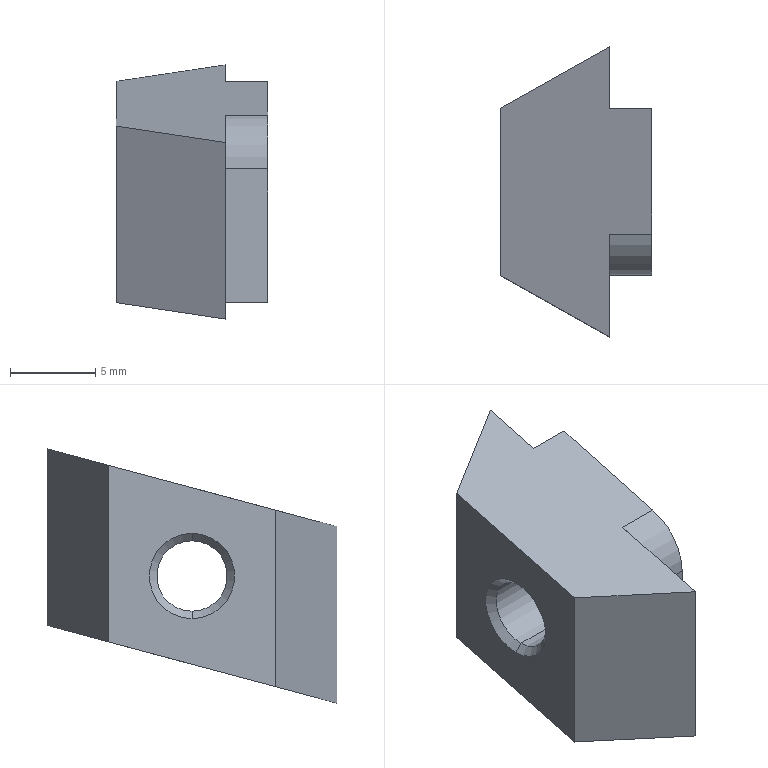Part | STEP file | 0245_012_HNTFSN8-5 | 1 solid | 18 faces | box 8.9 x 17 x 14.908 mm | volume 1013 mm3 | plane 10 | cone 4 | cylinder 4 | commonest cylinder face diameters 4.134 x2 6.533 x2
STEP:
#1=CARTESIAN_POINT('',(0.,0.,0.));
#2=DIRECTION('',(0.,0.,1.));
#3=DIRECTION('',(1.,0.,0.));
#4=AXIS2_PLACEMENT_3D('',#1,#2,#3);
#5=CARTESIAN_POINT('',(-8.467,0.,2.067));
#6=VERTEX_POINT('',#5);
#7=CARTESIAN_POINT('',(-8.9,0.,2.5));
#8=VERTEX_POINT('',#7);
#9=CARTESIAN_POINT('',(-8.9,0.,2.5));
#10=DIRECTION('',(-0.7071,0.,0.7071));
#11=VECTOR('',#10,1.);
#12=LINE('',#9,#11);
#13=CARTESIAN_POINT('',(-8.9,0.,0.));
#14=DIRECTION('',(-1.,0.,0.));
#15=DIRECTION('',(0.,0.,1.));
#16=AXIS2_PLACEMENT_3D('',#13,#14,#15);
#17=CONICAL_SURFACE('',#16,2.5,0.7854);
#18=CARTESIAN_POINT('',(6.283,0.));
#19=DIRECTION('',(0.,1.));
#20=VECTOR('',#19,1.);
#21=LINE('',#18,#20);
#22=(GEOMETRIC_REPRESENTATION_CONTEXT(2)PARAMETRIC_REPRESENTATION_CONTEXT()REPRESENTATION_CONTEXT('',''));
#23=DEFINITIONAL_REPRESENTATION('',(#21),#22);
#24=PCURVE('',#17,#23);
#25=CARTESIAN_POINT('',(-8.9,0.,0.));
#26=DIRECTION('',(-1.,0.,0.));
#27=DIRECTION('',(0.,0.,1.));
#28=AXIS2_PLACEMENT_3D('',#25,#26,#27);
#29=CONICAL_SURFACE('',#28,2.5,0.7854);
#30=CARTESIAN_POINT('',(0.,0.));
#31=DIRECTION('',(0.,1.));
#32=VECTOR('',#31,1.);
#33=LINE('',#30,#32);
#34=(GEOMETRIC_REPRESENTATION_CONTEXT(2)PARAMETRIC_REPRESENTATION_CONTEXT()REPRESENTATION_CONTEXT('',''));
#35=DEFINITIONAL_REPRESENTATION('',(#33),#34);
#36=PCURVE('',#29,#35);
#37=SURFACE_CURVE('',#12,(#24,#36),.PCURVE_S1.);
#38=EDGE_CURVE('',#6,#8,#37,.T.);
#39=ORIENTED_EDGE('',*,*,#38,.T.);
#40=CARTESIAN_POINT('',(-8.9,0.,-2.5));
#41=VERTEX_POINT('',#40);
#42=CARTESIAN_POINT('',(-8.9,0.,0.));
#43=DIRECTION('',(-1.,0.,0.));
#44=DIRECTION('',(0.,0.,1.));
#45=AXIS2_PLACEMENT_3D('',#42,#43,#44);
#46=CIRCLE('',#45,2.5);
#47=CARTESIAN_POINT('',(0.,0.));
#48=DIRECTION('',(1.,0.));
#49=VECTOR('',#48,1.);
#50=LINE('',#47,#49);
#51=(GEOMETRIC_REPRESENTATION_CONTEXT(2)PARAMETRIC_REPRESENTATION_CONTEXT()REPRESENTATION_CONTEXT('',''));
#52=DEFINITIONAL_REPRESENTATION('',(#50),#51);
#53=PCURVE('',#17,#52);
#54=CARTESIAN_POINT('',(-8.9,0.,0.));
#55=DIRECTION('',(1.,0.,0.));
#56=DIRECTION('',(0.,0.,-1.));
#57=AXIS2_PLACEMENT_3D('',#54,#55,#56);
#58=PLANE('',#57);
#59=CARTESIAN_POINT('',(-2.5,0.));
#60=CARTESIAN_POINT('',(-2.5,4.33));
#61=CARTESIAN_POINT('',(1.25,2.165));
#62=CARTESIAN_POINT('',(5.,0.));
#63=CARTESIAN_POINT('',(1.25,-2.165));
#64=CARTESIAN_POINT('',(-2.5,-4.33));
#65=CARTESIAN_POINT('',(-2.5,0.));
#66=(BOUNDED_CURVE()B_SPLINE_CURVE(2,(#59,#60,#61,#62,#63,#64,#65),.UNSPECIFIED.,.T.,.F.)B_SPLINE_CURVE_WITH_KNOTS((1,2,2,2,2,1),(-2.094,0.,2.094,4.189,6.283,8.378),.UNSPECIFIED.)CURVE()GEOMETRIC_REPRESENTATION_ITEM()RATIONAL_B_SPLINE_CURVE((1.,0.5,1.,0.5,1.,0.5,1.))REPRESENTATION_ITEM(''));
#67=(GEOMETRIC_REPRESENTATION_CONTEXT(2)PARAMETRIC_REPRESENTATION_CONTEXT()REPRESENTATION_CONTEXT('',''));
#68=DEFINITIONAL_REPRESENTATION('',(#66),#67);
#69=PCURVE('',#58,#68);
#70=SURFACE_CURVE('',#46,(#53,#69),.PCURVE_S1.);
#71=EDGE_CURVE('',#41,#8,#70,.T.);
#72=ORIENTED_EDGE('',*,*,#71,.F.);
#73=CARTESIAN_POINT('',(-8.467,0.,-2.067));
#74=VERTEX_POINT('',#73);
#75=CARTESIAN_POINT('',(-8.9,0.,-2.5));
#76=DIRECTION('',(-0.7071,0.,-0.7071));
#77=VECTOR('',#76,1.);
#78=LINE('',#75,#77);
#79=CARTESIAN_POINT('',(3.142,0.));
#80=DIRECTION('',(0.,1.));
#81=VECTOR('',#80,1.);
#82=LINE('',#79,#81);
#83=(GEOMETRIC_REPRESENTATION_CONTEXT(2)PARAMETRIC_REPRESENTATION_CONTEXT()REPRESENTATION_CONTEXT('',''));
#84=DEFINITIONAL_REPRESENTATION('',(#82),#83);
#85=PCURVE('',#17,#84);
#86=CARTESIAN_POINT('',(3.142,0.));
#87=DIRECTION('',(0.,1.));
#88=VECTOR('',#87,1.);
#89=LINE('',#86,#88);
#90=(GEOMETRIC_REPRESENTATION_CONTEXT(2)PARAMETRIC_REPRESENTATION_CONTEXT()REPRESENTATION_CONTEXT('',''));
#91=DEFINITIONAL_REPRESENTATION('',(#89),#90);
#92=PCURVE('',#29,#91);
#93=SURFACE_CURVE('',#78,(#85,#92),.PCURVE_S1.);
#94=EDGE_CURVE('',#74,#41,#93,.T.);
#95=ORIENTED_EDGE('',*,*,#94,.F.);
#96=CARTESIAN_POINT('',(-8.467,0.,0.));
#97=DIRECTION('',(-1.,0.,0.));
#98=DIRECTION('',(0.,1.,0.));
#99=AXIS2_PLACEMENT_3D('',#96,#97,#98);
#100=CIRCLE('',#99,2.067);
#101=CARTESIAN_POINT('',(1.571,-0.433));
#102=DIRECTION('',(1.,0.));
#103=VECTOR('',#102,1.);
#104=LINE('',#101,#103);
#105=(GEOMETRIC_REPRESENTATION_CONTEXT(2)PARAMETRIC_REPRESENTATION_CONTEXT()REPRESENTATION_CONTEXT('',''));
#106=DEFINITIONAL_REPRESENTATION('',(#104),#105);
#107=PCURVE('',#17,#106);
#108=CARTESIAN_POINT('',(-4.45,0.,0.));
#109=DIRECTION('',(1.,0.,0.));
#110=DIRECTION('',(0.,0.,-1.));
#111=AXIS2_PLACEMENT_3D('',#108,#109,#110);
#112=CYLINDRICAL_SURFACE('',#111,2.067);
#113=CARTESIAN_POINT('',(7.854,-4.017));
#114=DIRECTION('',(-1.,0.));
#115=VECTOR('',#114,1.);
#116=LINE('',#113,#115);
#117=(GEOMETRIC_REPRESENTATION_CONTEXT(2)PARAMETRIC_REPRESENTATION_CONTEXT()REPRESENTATION_CONTEXT('',''));
#118=DEFINITIONAL_REPRESENTATION('',(#116),#117);
#119=PCURVE('',#112,#118);
#120=SURFACE_CURVE('',#100,(#107,#119),.PCURVE_S1.);
#121=EDGE_CURVE('',#74,#6,#120,.T.);
#122=ORIENTED_EDGE('',*,*,#121,.T.);
#123=EDGE_LOOP('',(#39,#72,#95,#122));
#124=FACE_BOUND('',#123,.F.);
#125=ADVANCED_FACE('',(#124),#17,.F.);
#126=CARTESIAN_POINT('',(-0.433,0.,-2.067));
#127=VERTEX_POINT('',#126);
#128=CARTESIAN_POINT('',(0.,0.,-2.5));
#129=VERTEX_POINT('',#128);
#130=CARTESIAN_POINT('',(0.,0.,-2.5));
#131=DIRECTION('',(0.7071,0.,-0.7071));
#132=VECTOR('',#131,1.);
#133=LINE('',#130,#132);
#134=CARTESIAN_POINT('',(0.,0.,0.));
#135=DIRECTION('',(1.,0.,0.));
#136=DIRECTION('',(0.,0.,-1.));
#137=AXIS2_PLACEMENT_3D('',#134,#135,#136);
#138=CONICAL_SURFACE('',#137,2.5,0.7854);
#139=CARTESIAN_POINT('',(6.283,0.));
#140=DIRECTION('',(0.,1.));
#141=VECTOR('',#140,1.);
#142=LINE('',#139,#141);
#143=(GEOMETRIC_REPRESENTATION_CONTEXT(2)PARAMETRIC_REPRESENTATION_CONTEXT()REPRESENTATION_CONTEXT('',''));
#144=DEFINITIONAL_REPRESENTATION('',(#142),#143);
#145=PCURVE('',#138,#144);
#146=CARTESIAN_POINT('',(0.,0.,0.));
#147=DIRECTION('',(1.,0.,0.));
#148=DIRECTION('',(0.,0.,-1.));
#149=AXIS2_PLACEMENT_3D('',#146,#147,#148);
#150=CONICAL_SURFACE('',#149,2.5,0.7854);
#151=CARTESIAN_POINT('',(0.,0.));
#152=DIRECTION('',(0.,1.));
#153=VECTOR('',#152,1.);
#154=LINE('',#151,#153);
#155=(GEOMETRIC_REPRESENTATION_CONTEXT(2)PARAMETRIC_REPRESENTATION_CONTEXT()REPRESENTATION_CONTEXT('',''));
#156=DEFINITIONAL_REPRESENTATION('',(#154),#155);
#157=PCURVE('',#150,#156);
#158=SURFACE_CURVE('',#133,(#145,#157),.PCURVE_S1.);
#159=EDGE_CURVE('',#127,#129,#158,.T.);
#160=ORIENTED_EDGE('',*,*,#159,.T.);
#161=CARTESIAN_POINT('',(0.,0.,2.5));
#162=VERTEX_POINT('',#161);
#163=CARTESIAN_POINT('',(0.,0.,0.));
#164=DIRECTION('',(-1.,0.,0.));
#165=DIRECTION('',(0.,0.,-1.));
#166=AXIS2_PLACEMENT_3D('',#163,#164,#165);
#167=CIRCLE('',#166,2.5);
#168=CARTESIAN_POINT('',(6.283,0.));
#169=DIRECTION('',(-1.,0.));
#170=VECTOR('',#169,1.);
#171=LINE('',#168,#170);
#172=(GEOMETRIC_REPRESENTATION_CONTEXT(2)PARAMETRIC_REPRESENTATION_CONTEXT()REPRESENTATION_CONTEXT('',''));
#173=DEFINITIONAL_REPRESENTATION('',(#171),#172);
#174=PCURVE('',#138,#173);
#175=CARTESIAN_POINT('',(0.,0.,0.));
#176=DIRECTION('',(1.,0.,0.));
#177=DIRECTION('',(0.,0.,-1.));
#178=AXIS2_PLACEMENT_3D('',#175,#176,#177);
#179=PLANE('',#178);
#180=CARTESIAN_POINT('',(2.5,0.));
#181=CARTESIAN_POINT('',(2.5,-4.33));
#182=CARTESIAN_POINT('',(-1.25,-2.165));
#183=CARTESIAN_POINT('',(-5.,0.));
#184=CARTESIAN_POINT('',(-1.25,2.165));
#185=CARTESIAN_POINT('',(2.5,4.33));
#186=CARTESIAN_POINT('',(2.5,0.));
#187=(BOUNDED_CURVE()B_SPLINE_CURVE(2,(#180,#181,#182,#183,#184,#185,#186),.UNSPECIFIED.,.T.,.F.)B_SPLINE_CURVE_WITH_KNOTS((1,2,2,2,2,1),(-2.094,0.,2.094,4.189,6.283,8.378),.UNSPECIFIED.)CURVE()GEOMETRIC_REPRESENTATION_ITEM()RATIONAL_B_SPLINE_CURVE((1.,0.5,1.,0.5,1.,0.5,1.))REPRESENTATION_ITEM(''));
#188=(GEOMETRIC_REPRESENTATION_CONTEXT(2)PARAMETRIC_REPRESENTATION_CONTEXT()REPRESENTATION_CONTEXT('',''));
#189=DEFINITIONAL_REPRESENTATION('',(#187),#188);
#190=PCURVE('',#179,#189);
#191=SURFACE_CURVE('',#167,(#174,#190),.PCURVE_S1.);
#192=EDGE_CURVE('',#129,#162,#191,.T.);
#193=ORIENTED_EDGE('',*,*,#192,.T.);
#194=CARTESIAN_POINT('',(-0.433,0.,2.067));
#195=VERTEX_POINT('',#194);
#196=CARTESIAN_POINT('',(0.,0.,2.5));
#197=DIRECTION('',(0.7071,0.,0.7071));
#198=VECTOR('',#197,1.);
#199=LINE('',#196,#198);
#200=CARTESIAN_POINT('',(3.142,0.));
#201=DIRECTION('',(0.,1.));
#202=VECTOR('',#201,1.);
#203=LINE('',#200,#202);
#204=(GEOMETRIC_REPRESENTATION_CONTEXT(2)PARAMETRIC_REPRESENTATION_CONTEXT()REPRESENTATION_CONTEXT('',''));
#205=DEFINITIONAL_REPRESENTATION('',(#203),#204);
#206=PCURVE('',#138,#205);
#207=CARTESIAN_POINT('',(3.142,0.));
#208=DIRECTION('',(0.,1.));
#209=VECTOR('',#208,1.);
#210=LINE('',#207,#209);
#211=(GEOMETRIC_REPRESENTATION_CONTEXT(2)PARAMETRIC_REPRESENTATION_CONTEXT()REPRESENTATION_CONTEXT('',''));
#212=DEFINITIONAL_REPRESENTATION('',(#210),#211);
#213=PCURVE('',#150,#212);
#214=SURFACE_CURVE('',#199,(#206,#213),.PCURVE_S1.);
#215=EDGE_CURVE('',#195,#162,#214,.T.);
#216=ORIENTED_EDGE('',*,*,#215,.F.);
#217=CARTESIAN_POINT('',(-0.433,0.,0.));
#218=DIRECTION('',(1.,0.,0.));
#219=DIRECTION('',(0.,1.,0.));
#220=AXIS2_PLACEMENT_3D('',#217,#218,#219);
#221=CIRCLE('',#220,2.067);
#222=CARTESIAN_POINT('',(1.571,-0.433));
#223=DIRECTION('',(1.,0.));
#224=VECTOR('',#223,1.);
#225=LINE('',#222,#224);
#226=(GEOMETRIC_REPRESENTATION_CONTEXT(2)PARAMETRIC_REPRESENTATION_CONTEXT()REPRESENTATION_CONTEXT('',''));
#227=DEFINITIONAL_REPRESENTATION('',(#225),#226);
#228=PCURVE('',#138,#227);
#229=CARTESIAN_POINT('',(1.571,4.017));
#230=DIRECTION('',(1.,0.));
#231=VECTOR('',#230,1.);
#232=LINE('',#229,#231);
#233=(GEOMETRIC_REPRESENTATION_CONTEXT(2)PARAMETRIC_REPRESENTATION_CONTEXT()REPRESENTATION_CONTEXT('',''));
#234=DEFINITIONAL_REPRESENTATION('',(#232),#233);
#235=PCURVE('',#112,#234);
#236=SURFACE_CURVE('',#221,(#228,#235),.PCURVE_S1.);
#237=EDGE_CURVE('',#195,#127,#236,.T.);
#238=ORIENTED_EDGE('',*,*,#237,.T.);
#239=EDGE_LOOP('',(#160,#193,#216,#238));
#240=FACE_BOUND('',#239,.F.);
#241=ADVANCED_FACE('',(#240),#138,.F.);
#242=CARTESIAN_POINT('',(-4.45,0.,-2.067));
#243=DIRECTION('',(1.,0.,0.));
#244=VECTOR('',#243,1.);
#245=LINE('',#242,#244);
#246=CARTESIAN_POINT('',(6.283,0.));
#247=DIRECTION('',(0.,1.));
#248=VECTOR('',#247,1.);
#249=LINE('',#246,#248);
#250=(GEOMETRIC_REPRESENTATION_CONTEXT(2)PARAMETRIC_REPRESENTATION_CONTEXT()REPRESENTATION_CONTEXT('',''));
#251=DEFINITIONAL_REPRESENTATION('',(#249),#250);
#252=PCURVE('',#112,#251);
#253=CARTESIAN_POINT('',(-4.45,0.,0.));
#254=DIRECTION('',(1.,0.,0.));
#255=DIRECTION('',(0.,0.,-1.));
#256=AXIS2_PLACEMENT_3D('',#253,#254,#255);
#257=CYLINDRICAL_SURFACE('',#256,2.067);
#258=CARTESIAN_POINT('',(0.,0.));
#259=DIRECTION('',(0.,1.));
#260=VECTOR('',#259,1.);
#261=LINE('',#258,#260);
#262=(GEOMETRIC_REPRESENTATION_CONTEXT(2)PARAMETRIC_REPRESENTATION_CONTEXT()REPRESENTATION_CONTEXT('',''));
#263=DEFINITIONAL_REPRESENTATION('',(#261),#262);
#264=PCURVE('',#257,#263);
#265=SURFACE_CURVE('',#245,(#252,#264),.PCURVE_S1.);
#266=EDGE_CURVE('',#74,#127,#265,.T.);
#267=ORIENTED_EDGE('',*,*,#266,.T.);
#268=ORIENTED_EDGE('',*,*,#237,.F.);
#269=CARTESIAN_POINT('',(-4.45,0.,2.067));
#270=DIRECTION('',(1.,0.,0.));
#271=VECTOR('',#270,1.);
#272=LINE('',#269,#271);
#273=CARTESIAN_POINT('',(3.142,0.));
#274=DIRECTION('',(0.,1.));
#275=VECTOR('',#274,1.);
#276=LINE('',#273,#275);
#277=(GEOMETRIC_REPRESENTATION_CONTEXT(2)PARAMETRIC_REPRESENTATION_CONTEXT()REPRESENTATION_CONTEXT('',''));
#278=DEFINITIONAL_REPRESENTATION('',(#276),#277);
#279=PCURVE('',#112,#278);
#280=CARTESIAN_POINT('',(3.142,0.));
#281=DIRECTION('',(0.,1.));
#282=VECTOR('',#281,1.);
#283=LINE('',#280,#282);
#284=(GEOMETRIC_REPRESENTATION_CONTEXT(2)PARAMETRIC_REPRESENTATION_CONTEXT()REPRESENTATION_CONTEXT('',''));
#285=DEFINITIONAL_REPRESENTATION('',(#283),#284);
#286=PCURVE('',#257,#285);
#287=SURFACE_CURVE('',#272,(#279,#286),.PCURVE_S1.);
#288=EDGE_CURVE('',#6,#195,#287,.T.);
#289=ORIENTED_EDGE('',*,*,#288,.F.);
#290=ORIENTED_EDGE('',*,*,#121,.F.);
#291=EDGE_LOOP('',(#267,#268,#289,#290));
#292=FACE_BOUND('',#291,.F.);
#293=ADVANCED_FACE('',(#292),#112,.F.);
#294=CARTESIAN_POINT('',(-8.9,-4.9,3.863));
#295=VERTEX_POINT('',#294);
#296=CARTESIAN_POINT('',(-2.5,-8.5,2.899));
#297=VERTEX_POINT('',#296);
#298=CARTESIAN_POINT('',(-8.9,-4.9,3.863));
#299=DIRECTION('',(0.8642,-0.4861,-0.1302));
#300=VECTOR('',#299,1.);
#301=LINE('',#298,#300);
#302=CARTESIAN_POINT('',(0.,8.5,7.454));
#303=DIRECTION('',(0.,-0.2588,0.9659));
#304=DIRECTION('',(0.,-0.9659,-0.2588));
#305=AXIS2_PLACEMENT_3D('',#302,#303,#304);
#306=PLANE('',#305);
#307=CARTESIAN_POINT('',(13.873,-8.9));
#308=DIRECTION('',(0.5032,0.8642));
#309=VECTOR('',#308,1.);
#310=LINE('',#307,#309);
#311=(GEOMETRIC_REPRESENTATION_CONTEXT(2)PARAMETRIC_REPRESENTATION_CONTEXT()REPRESENTATION_CONTEXT('',''));
#312=DEFINITIONAL_REPRESENTATION('',(#310),#311);
#313=PCURVE('',#306,#312);
#314=CARTESIAN_POINT('',(-2.5,-8.5,20.));
#315=DIRECTION('',(0.4903,0.8716,0.));
#316=DIRECTION('',(-0.8716,0.4903,0.));
#317=AXIS2_PLACEMENT_3D('',#314,#315,#316);
#318=PLANE('',#317);
#319=CARTESIAN_POINT('',(7.343,-16.137));
#320=DIRECTION('',(-0.9915,-0.1302));
#321=VECTOR('',#320,1.);
#322=LINE('',#319,#321);
#323=(GEOMETRIC_REPRESENTATION_CONTEXT(2)PARAMETRIC_REPRESENTATION_CONTEXT()REPRESENTATION_CONTEXT('',''));
#324=DEFINITIONAL_REPRESENTATION('',(#322),#323);
#325=PCURVE('',#318,#324);
#326=SURFACE_CURVE('',#301,(#313,#325),.PCURVE_S1.);
#327=EDGE_CURVE('',#295,#297,#326,.T.);
#328=ORIENTED_EDGE('',*,*,#327,.T.);
#329=CARTESIAN_POINT('',(-2.5,-2.479,4.512));
#330=VERTEX_POINT('',#329);
#331=CARTESIAN_POINT('',(-2.5,8.5,7.454));
#332=DIRECTION('',(0.,0.9659,0.2588));
#333=VECTOR('',#332,1.);
#334=LINE('',#331,#333);
#335=CARTESIAN_POINT('',(0.,-2.5));
#336=DIRECTION('',(-1.,0.));
#337=VECTOR('',#336,1.);
#338=LINE('',#335,#337);
#339=(GEOMETRIC_REPRESENTATION_CONTEXT(2)PARAMETRIC_REPRESENTATION_CONTEXT()REPRESENTATION_CONTEXT('',''));
#340=DEFINITIONAL_REPRESENTATION('',(#338),#339);
#341=PCURVE('',#306,#340);
#342=CARTESIAN_POINT('',(-2.5,-4.9,20.));
#343=DIRECTION('',(-1.,0.,0.));
#344=DIRECTION('',(0.,0.,1.));
#345=AXIS2_PLACEMENT_3D('',#342,#343,#344);
#346=PLANE('',#345);
#347=CARTESIAN_POINT('',(-12.546,13.4));
#348=DIRECTION('',(0.2588,0.9659));
#349=VECTOR('',#348,1.);
#350=LINE('',#347,#349);
#351=(GEOMETRIC_REPRESENTATION_CONTEXT(2)PARAMETRIC_REPRESENTATION_CONTEXT()REPRESENTATION_CONTEXT('',''));
#352=DEFINITIONAL_REPRESENTATION('',(#350),#351);
#353=PCURVE('',#346,#352);
#354=SURFACE_CURVE('',#334,(#341,#353),.PCURVE_S1.);
#355=EDGE_CURVE('',#297,#330,#354,.T.);
#356=ORIENTED_EDGE('',*,*,#355,.T.);
#357=CARTESIAN_POINT('',(0.,-2.479,4.512));
#358=VERTEX_POINT('',#357);
#359=CARTESIAN_POINT('',(0.,-2.479,4.512));
#360=DIRECTION('',(1.,0.,0.));
#361=VECTOR('',#360,1.);
#362=LINE('',#359,#361);
#363=CARTESIAN_POINT('',(11.366,0.));
#364=DIRECTION('',(0.,1.));
#365=VECTOR('',#364,1.);
#366=LINE('',#363,#365);
#367=(GEOMETRIC_REPRESENTATION_CONTEXT(2)PARAMETRIC_REPRESENTATION_CONTEXT()REPRESENTATION_CONTEXT('',''));
#368=DEFINITIONAL_REPRESENTATION('',(#366),#367);
#369=PCURVE('',#306,#368);
#370=CARTESIAN_POINT('',(-2.5,-1.633,1.357));
#371=DIRECTION('',(-1.,0.,0.));
#372=DIRECTION('',(0.,0.,1.));
#373=AXIS2_PLACEMENT_3D('',#370,#371,#372);
#374=CYLINDRICAL_SURFACE('',#373,3.267);
#375=CARTESIAN_POINT('',(6.021,-2.5));
#376=DIRECTION('',(0.,-1.));
#377=VECTOR('',#376,1.);
#378=LINE('',#375,#377);
#379=(GEOMETRIC_REPRESENTATION_CONTEXT(2)PARAMETRIC_REPRESENTATION_CONTEXT()REPRESENTATION_CONTEXT('',''));
#380=DEFINITIONAL_REPRESENTATION('',(#378),#379);
#381=PCURVE('',#374,#380);
#382=SURFACE_CURVE('',#362,(#369,#381),.PCURVE_S1.);
#383=EDGE_CURVE('',#330,#358,#382,.T.);
#384=ORIENTED_EDGE('',*,*,#383,.T.);
#385=CARTESIAN_POINT('',(0.,4.9,6.489));
#386=VERTEX_POINT('',#385);
#387=CARTESIAN_POINT('',(0.,8.5,7.454));
#388=DIRECTION('',(0.,0.9659,0.2588));
#389=VECTOR('',#388,1.);
#390=LINE('',#387,#389);
#391=CARTESIAN_POINT('',(0.,0.));
#392=DIRECTION('',(-1.,0.));
#393=VECTOR('',#392,1.);
#394=LINE('',#391,#393);
#395=(GEOMETRIC_REPRESENTATION_CONTEXT(2)PARAMETRIC_REPRESENTATION_CONTEXT()REPRESENTATION_CONTEXT('',''));
#396=DEFINITIONAL_REPRESENTATION('',(#394),#395);
#397=PCURVE('',#306,#396);
#398=CARTESIAN_POINT('',(-7.454,8.5));
#399=DIRECTION('',(-0.2588,0.9659));
#400=VECTOR('',#399,1.);
#401=LINE('',#398,#400);
#402=(GEOMETRIC_REPRESENTATION_CONTEXT(2)PARAMETRIC_REPRESENTATION_CONTEXT()REPRESENTATION_CONTEXT('',''));
#403=DEFINITIONAL_REPRESENTATION('',(#401),#402);
#404=PCURVE('',#179,#403);
#405=SURFACE_CURVE('',#390,(#397,#404),.PCURVE_S1.);
#406=EDGE_CURVE('',#358,#386,#405,.T.);
#407=ORIENTED_EDGE('',*,*,#406,.T.);
#408=CARTESIAN_POINT('',(-2.5,4.9,6.489));
#409=VERTEX_POINT('',#408);
#410=CARTESIAN_POINT('',(0.,4.9,6.489));
#411=DIRECTION('',(-1.,0.,0.));
#412=VECTOR('',#411,1.);
#413=LINE('',#410,#412);
#414=CARTESIAN_POINT('',(3.727,0.));
#415=DIRECTION('',(0.,-1.));
#416=VECTOR('',#415,1.);
#417=LINE('',#414,#416);
#418=(GEOMETRIC_REPRESENTATION_CONTEXT(2)PARAMETRIC_REPRESENTATION_CONTEXT()REPRESENTATION_CONTEXT('',''));
#419=DEFINITIONAL_REPRESENTATION('',(#417),#418);
#420=PCURVE('',#306,#419);
#421=CARTESIAN_POINT('',(-2.5,4.9,20.));
#422=DIRECTION('',(0.,-1.,0.));
#423=DIRECTION('',(1.,0.,0.));
#424=AXIS2_PLACEMENT_3D('',#421,#422,#423);
#425=PLANE('',#424);
#426=CARTESIAN_POINT('',(2.5,-13.511));
#427=DIRECTION('',(-1.,0.));
#428=VECTOR('',#427,1.);
#429=LINE('',#426,#428);
#430=(GEOMETRIC_REPRESENTATION_CONTEXT(2)PARAMETRIC_REPRESENTATION_CONTEXT()REPRESENTATION_CONTEXT('',''));
#431=DEFINITIONAL_REPRESENTATION('',(#429),#430);
#432=PCURVE('',#425,#431);
#433=SURFACE_CURVE('',#413,(#420,#432),.PCURVE_S1.);
#434=EDGE_CURVE('',#386,#409,#433,.T.);
#435=ORIENTED_EDGE('',*,*,#434,.T.);
#436=CARTESIAN_POINT('',(-2.5,8.5,7.454));
#437=VERTEX_POINT('',#436);
#438=CARTESIAN_POINT('',(-2.5,8.5,7.454));
#439=DIRECTION('',(0.,0.9659,0.2588));
#440=VECTOR('',#439,1.);
#441=LINE('',#438,#440);
#442=CARTESIAN_POINT('',(0.,-2.5));
#443=DIRECTION('',(-1.,0.));
#444=VECTOR('',#443,1.);
#445=LINE('',#442,#444);
#446=(GEOMETRIC_REPRESENTATION_CONTEXT(2)PARAMETRIC_REPRESENTATION_CONTEXT()REPRESENTATION_CONTEXT('',''));
#447=DEFINITIONAL_REPRESENTATION('',(#445),#446);
#448=PCURVE('',#306,#447);
#449=CARTESIAN_POINT('',(-2.5,8.5,20.));
#450=DIRECTION('',(-1.,0.,0.));
#451=DIRECTION('',(0.,0.,1.));
#452=AXIS2_PLACEMENT_3D('',#449,#450,#451);
#453=PLANE('',#452);
#454=CARTESIAN_POINT('',(-12.546,0.));
#455=DIRECTION('',(0.2588,0.9659));
#456=VECTOR('',#455,1.);
#457=LINE('',#454,#456);
#458=(GEOMETRIC_REPRESENTATION_CONTEXT(2)PARAMETRIC_REPRESENTATION_CONTEXT()REPRESENTATION_CONTEXT('',''));
#459=DEFINITIONAL_REPRESENTATION('',(#457),#458);
#460=PCURVE('',#453,#459);
#461=SURFACE_CURVE('',#441,(#448,#460),.PCURVE_S1.);
#462=EDGE_CURVE('',#409,#437,#461,.T.);
#463=ORIENTED_EDGE('',*,*,#462,.T.);
#464=CARTESIAN_POINT('',(-8.9,4.9,6.489));
#465=VERTEX_POINT('',#464);
#466=CARTESIAN_POINT('',(-2.5,8.5,7.454));
#467=DIRECTION('',(-0.8642,-0.4861,-0.1302));
#468=VECTOR('',#467,1.);
#469=LINE('',#466,#468);
#470=CARTESIAN_POINT('',(0.,-2.5));
#471=DIRECTION('',(0.5032,-0.8642));
#472=VECTOR('',#471,1.);
#473=LINE('',#470,#472);
#474=(GEOMETRIC_REPRESENTATION_CONTEXT(2)PARAMETRIC_REPRESENTATION_CONTEXT()REPRESENTATION_CONTEXT('',''));
#475=DEFINITIONAL_REPRESENTATION('',(#473),#474);
#476=PCURVE('',#306,#475);
#477=CARTESIAN_POINT('',(-8.9,4.9,20.));
#478=DIRECTION('',(0.4903,-0.8716,0.));
#479=DIRECTION('',(0.8716,0.4903,0.));
#480=AXIS2_PLACEMENT_3D('',#477,#478,#479);
#481=PLANE('',#480);
#482=CARTESIAN_POINT('',(7.343,-12.546));
#483=DIRECTION('',(-0.9915,-0.1302));
#484=VECTOR('',#483,1.);
#485=LINE('',#482,#484);
#486=(GEOMETRIC_REPRESENTATION_CONTEXT(2)PARAMETRIC_REPRESENTATION_CONTEXT()REPRESENTATION_CONTEXT('',''));
#487=DEFINITIONAL_REPRESENTATION('',(#485),#486);
#488=PCURVE('',#481,#487);
#489=SURFACE_CURVE('',#469,(#476,#488),.PCURVE_S1.);
#490=EDGE_CURVE('',#437,#465,#489,.T.);
#491=ORIENTED_EDGE('',*,*,#490,.T.);
#492=CARTESIAN_POINT('',(-8.9,8.5,7.454));
#493=DIRECTION('',(0.,-0.9659,-0.2588));
#494=VECTOR('',#493,1.);
#495=LINE('',#492,#494);
#496=CARTESIAN_POINT('',(0.,-8.9));
#497=DIRECTION('',(1.,0.));
#498=VECTOR('',#497,1.);
#499=LINE('',#496,#498);
#500=(GEOMETRIC_REPRESENTATION_CONTEXT(2)PARAMETRIC_REPRESENTATION_CONTEXT()REPRESENTATION_CONTEXT('',''));
#501=DEFINITIONAL_REPRESENTATION('',(#499),#500);
#502=PCURVE('',#306,#501);
#503=CARTESIAN_POINT('',(-7.454,8.5));
#504=DIRECTION('',(0.2588,-0.9659));
#505=VECTOR('',#504,1.);
#506=LINE('',#503,#505);
#507=(GEOMETRIC_REPRESENTATION_CONTEXT(2)PARAMETRIC_REPRESENTATION_CONTEXT()REPRESENTATION_CONTEXT('',''));
#508=DEFINITIONAL_REPRESENTATION('',(#506),#507);
#509=PCURVE('',#58,#508);
#510=SURFACE_CURVE('',#495,(#502,#509),.PCURVE_S1.);
#511=EDGE_CURVE('',#465,#295,#510,.T.);
#512=ORIENTED_EDGE('',*,*,#511,.T.);
#513=EDGE_LOOP('',(#328,#356,#384,#407,#435,#463,#491,#512));
#514=FACE_BOUND('',#513,.T.);
#515=ADVANCED_FACE('',(#514),#306,.T.);
#516=CARTESIAN_POINT('',(-2.5,-8.5,-7.454));
#517=VERTEX_POINT('',#516);
#518=CARTESIAN_POINT('',(-2.5,-8.5,20.));
#519=DIRECTION('',(0.,0.,1.));
#520=VECTOR('',#519,1.);
#521=LINE('',#518,#520);
#522=CARTESIAN_POINT('',(0.,-3.6));
#523=DIRECTION('',(1.,0.));
#524=VECTOR('',#523,1.);
#525=LINE('',#522,#524);
#526=(GEOMETRIC_REPRESENTATION_CONTEXT(2)PARAMETRIC_REPRESENTATION_CONTEXT()REPRESENTATION_CONTEXT('',''));
#527=DEFINITIONAL_REPRESENTATION('',(#525),#526);
#528=PCURVE('',#346,#527);
#529=CARTESIAN_POINT('',(0.,0.));
#530=DIRECTION('',(0.,1.));
#531=VECTOR('',#530,1.);
#532=LINE('',#529,#531);
#533=(GEOMETRIC_REPRESENTATION_CONTEXT(2)PARAMETRIC_REPRESENTATION_CONTEXT()REPRESENTATION_CONTEXT('',''));
#534=DEFINITIONAL_REPRESENTATION('',(#532),#533);
#535=PCURVE('',#318,#534);
#536=SURFACE_CURVE('',#521,(#528,#535),.PCURVE_S1.);
#537=EDGE_CURVE('',#517,#297,#536,.T.);
#538=ORIENTED_EDGE('',*,*,#537,.F.);
#539=CARTESIAN_POINT('',(-2.5,-4.9,-6.489));
#540=VERTEX_POINT('',#539);
#541=CARTESIAN_POINT('',(-2.5,-4.9,-6.489));
#542=DIRECTION('',(0.,-0.9659,-0.2588));
#543=VECTOR('',#542,1.);
#544=LINE('',#541,#543);
#545=CARTESIAN_POINT('',(-26.489,0.));
#546=DIRECTION('',(-0.2588,-0.9659));
#547=VECTOR('',#546,1.);
#548=LINE('',#545,#547);
#549=(GEOMETRIC_REPRESENTATION_CONTEXT(2)PARAMETRIC_REPRESENTATION_CONTEXT()REPRESENTATION_CONTEXT('',''));
#550=DEFINITIONAL_REPRESENTATION('',(#548),#549);
#551=PCURVE('',#346,#550);
#552=CARTESIAN_POINT('',(0.,-8.5,-7.454));
#553=DIRECTION('',(0.,0.2588,-0.9659));
#554=DIRECTION('',(0.,0.9659,0.2588));
#555=AXIS2_PLACEMENT_3D('',#552,#553,#554);
#556=PLANE('',#555);
#557=CARTESIAN_POINT('',(3.727,-2.5));
#558=DIRECTION('',(-1.,0.));
#559=VECTOR('',#558,1.);
#560=LINE('',#557,#559);
#561=(GEOMETRIC_REPRESENTATION_CONTEXT(2)PARAMETRIC_REPRESENTATION_CONTEXT()REPRESENTATION_CONTEXT('',''));
#562=DEFINITIONAL_REPRESENTATION('',(#560),#561);
#563=PCURVE('',#556,#562);
#564=SURFACE_CURVE('',#544,(#551,#563),.PCURVE_S1.);
#565=EDGE_CURVE('',#540,#517,#564,.T.);
#566=ORIENTED_EDGE('',*,*,#565,.F.);
#567=CARTESIAN_POINT('',(-2.5,-4.9,1.357));
#568=VERTEX_POINT('',#567);
#569=CARTESIAN_POINT('',(-2.5,-4.9,20.));
#570=DIRECTION('',(0.,0.,-1.));
#571=VECTOR('',#570,1.);
#572=LINE('',#569,#571);
#573=CARTESIAN_POINT('',(0.,0.));
#574=DIRECTION('',(-1.,0.));
#575=VECTOR('',#574,1.);
#576=LINE('',#573,#575);
#577=(GEOMETRIC_REPRESENTATION_CONTEXT(2)PARAMETRIC_REPRESENTATION_CONTEXT()REPRESENTATION_CONTEXT('',''));
#578=DEFINITIONAL_REPRESENTATION('',(#576),#577);
#579=PCURVE('',#346,#578);
#580=CARTESIAN_POINT('',(0.,-4.9,20.));
#581=DIRECTION('',(0.,1.,0.));
#582=DIRECTION('',(-1.,0.,0.));
#583=AXIS2_PLACEMENT_3D('',#580,#581,#582);
#584=PLANE('',#583);
#585=CARTESIAN_POINT('',(2.5,0.));
#586=DIRECTION('',(0.,-1.));
#587=VECTOR('',#586,1.);
#588=LINE('',#585,#587);
#589=(GEOMETRIC_REPRESENTATION_CONTEXT(2)PARAMETRIC_REPRESENTATION_CONTEXT()REPRESENTATION_CONTEXT('',''));
#590=DEFINITIONAL_REPRESENTATION('',(#588),#589);
#591=PCURVE('',#584,#590);
#592=SURFACE_CURVE('',#572,(#579,#591),.PCURVE_S1.);
#593=EDGE_CURVE('',#568,#540,#592,.T.);
#594=ORIENTED_EDGE('',*,*,#593,.F.);
#595=CARTESIAN_POINT('',(-2.5,-1.633,1.357));
#596=DIRECTION('',(1.,0.,0.));
#597=DIRECTION('',(0.,0.,1.));
#598=AXIS2_PLACEMENT_3D('',#595,#596,#597);
#599=CIRCLE('',#598,3.267);
#600=CARTESIAN_POINT('',(-15.377,3.267));
#601=CARTESIAN_POINT('',(-15.377,-2.391));
#602=CARTESIAN_POINT('',(-20.277,0.4377));
#603=CARTESIAN_POINT('',(-25.177,3.267));
#604=CARTESIAN_POINT('',(-20.277,6.096));
#605=CARTESIAN_POINT('',(-15.377,8.925));
#606=CARTESIAN_POINT('',(-15.377,3.267));
#607=(BOUNDED_CURVE()B_SPLINE_CURVE(2,(#600,#601,#602,#603,#604,#605,#606),.UNSPECIFIED.,.T.,.F.)B_SPLINE_CURVE_WITH_KNOTS((1,2,2,2,2,1),(-2.094,0.,2.094,4.189,6.283,8.378),.UNSPECIFIED.)CURVE()GEOMETRIC_REPRESENTATION_ITEM()RATIONAL_B_SPLINE_CURVE((1.,0.5,1.,0.5,1.,0.5,1.))REPRESENTATION_ITEM(''));
#608=(GEOMETRIC_REPRESENTATION_CONTEXT(2)PARAMETRIC_REPRESENTATION_CONTEXT()REPRESENTATION_CONTEXT('',''));
#609=DEFINITIONAL_REPRESENTATION('',(#607),#608);
#610=PCURVE('',#346,#609);
#611=CARTESIAN_POINT('',(6.283,0.));
#612=DIRECTION('',(-1.,0.));
#613=VECTOR('',#612,1.);
#614=LINE('',#611,#613);
#615=(GEOMETRIC_REPRESENTATION_CONTEXT(2)PARAMETRIC_REPRESENTATION_CONTEXT()REPRESENTATION_CONTEXT('',''));
#616=DEFINITIONAL_REPRESENTATION('',(#614),#615);
#617=PCURVE('',#374,#616);
#618=SURFACE_CURVE('',#599,(#610,#617),.PCURVE_S1.);
#619=EDGE_CURVE('',#330,#568,#618,.T.);
#620=ORIENTED_EDGE('',*,*,#619,.F.);
#621=ORIENTED_EDGE('',*,*,#355,.F.);
#622=EDGE_LOOP('',(#538,#566,#594,#620,#621));
#623=FACE_BOUND('',#622,.T.);
#624=ADVANCED_FACE('',(#623),#346,.F.);
#625=ORIENTED_EDGE('',*,*,#537,.T.);
#626=ORIENTED_EDGE('',*,*,#327,.F.);
#627=CARTESIAN_POINT('',(-8.9,-4.9,-6.489));
#628=VERTEX_POINT('',#627);
#629=CARTESIAN_POINT('',(-8.9,-4.9,20.));
#630=DIRECTION('',(0.,0.,1.));
#631=VECTOR('',#630,1.);
#632=LINE('',#629,#631);
#633=CARTESIAN_POINT('',(7.343,0.));
#634=DIRECTION('',(0.,1.));
#635=VECTOR('',#634,1.);
#636=LINE('',#633,#635);
#637=(GEOMETRIC_REPRESENTATION_CONTEXT(2)PARAMETRIC_REPRESENTATION_CONTEXT()REPRESENTATION_CONTEXT('',''));
#638=DEFINITIONAL_REPRESENTATION('',(#636),#637);
#639=PCURVE('',#318,#638);
#640=CARTESIAN_POINT('',(-20.,-4.9));
#641=DIRECTION('',(-1.,0.));
#642=VECTOR('',#641,1.);
#643=LINE('',#640,#642);
#644=(GEOMETRIC_REPRESENTATION_CONTEXT(2)PARAMETRIC_REPRESENTATION_CONTEXT()REPRESENTATION_CONTEXT('',''));
#645=DEFINITIONAL_REPRESENTATION('',(#643),#644);
#646=PCURVE('',#58,#645);
#647=SURFACE_CURVE('',#632,(#639,#646),.PCURVE_S1.);
#648=EDGE_CURVE('',#628,#295,#647,.T.);
#649=ORIENTED_EDGE('',*,*,#648,.F.);
#650=CARTESIAN_POINT('',(-2.5,-8.5,-7.454));
#651=DIRECTION('',(-0.8642,0.4861,0.1302));
#652=VECTOR('',#651,1.);
#653=LINE('',#650,#652);
#654=CARTESIAN_POINT('',(0.,-27.454));
#655=DIRECTION('',(0.9915,0.1302));
#656=VECTOR('',#655,1.);
#657=LINE('',#654,#656);
#658=(GEOMETRIC_REPRESENTATION_CONTEXT(2)PARAMETRIC_REPRESENTATION_CONTEXT()REPRESENTATION_CONTEXT('',''));
#659=DEFINITIONAL_REPRESENTATION('',(#657),#658);
#660=PCURVE('',#318,#659);
#661=CARTESIAN_POINT('',(0.,-2.5));
#662=DIRECTION('',(0.5032,-0.8642));
#663=VECTOR('',#662,1.);
#664=LINE('',#661,#663);
#665=(GEOMETRIC_REPRESENTATION_CONTEXT(2)PARAMETRIC_REPRESENTATION_CONTEXT()REPRESENTATION_CONTEXT('',''));
#666=DEFINITIONAL_REPRESENTATION('',(#664),#665);
#667=PCURVE('',#556,#666);
#668=SURFACE_CURVE('',#653,(#660,#667),.PCURVE_S1.);
#669=EDGE_CURVE('',#517,#628,#668,.T.);
#670=ORIENTED_EDGE('',*,*,#669,.F.);
#671=EDGE_LOOP('',(#625,#626,#649,#670));
#672=FACE_BOUND('',#671,.T.);
#673=ADVANCED_FACE('',(#672),#318,.F.);
#674=CARTESIAN_POINT('',(-8.9,4.9,-3.863));
#675=VERTEX_POINT('',#674);
#676=CARTESIAN_POINT('',(-8.9,-4.9,-6.489));
#677=DIRECTION('',(0.,0.9659,0.2588));
#678=VECTOR('',#677,1.);
#679=LINE('',#676,#678);
#680=CARTESIAN_POINT('',(6.489,-4.9));
#681=DIRECTION('',(-0.2588,0.9659));
#682=VECTOR('',#681,1.);
#683=LINE('',#680,#682);
#684=(GEOMETRIC_REPRESENTATION_CONTEXT(2)PARAMETRIC_REPRESENTATION_CONTEXT()REPRESENTATION_CONTEXT('',''));
#685=DEFINITIONAL_REPRESENTATION('',(#683),#684);
#686=PCURVE('',#58,#685);
#687=CARTESIAN_POINT('',(3.727,-8.9));
#688=DIRECTION('',(1.,0.));
#689=VECTOR('',#688,1.);
#690=LINE('',#687,#689);
#691=(GEOMETRIC_REPRESENTATION_CONTEXT(2)PARAMETRIC_REPRESENTATION_CONTEXT()REPRESENTATION_CONTEXT('',''));
#692=DEFINITIONAL_REPRESENTATION('',(#690),#691);
#693=PCURVE('',#556,#692);
#694=SURFACE_CURVE('',#679,(#686,#693),.PCURVE_S1.);
#695=EDGE_CURVE('',#628,#675,#694,.T.);
#696=ORIENTED_EDGE('',*,*,#695,.F.);
#697=ORIENTED_EDGE('',*,*,#648,.T.);
#698=ORIENTED_EDGE('',*,*,#511,.F.);
#699=CARTESIAN_POINT('',(-8.9,4.9,0.));
#700=DIRECTION('',(0.,0.,1.));
#701=VECTOR('',#700,1.);
#702=LINE('',#699,#701);
#703=CARTESIAN_POINT('',(0.,4.9));
#704=DIRECTION('',(-1.,0.));
#705=VECTOR('',#704,1.);
#706=LINE('',#703,#705);
#707=(GEOMETRIC_REPRESENTATION_CONTEXT(2)PARAMETRIC_REPRESENTATION_CONTEXT()REPRESENTATION_CONTEXT('',''));
#708=DEFINITIONAL_REPRESENTATION('',(#706),#707);
#709=PCURVE('',#58,#708);
#710=CARTESIAN_POINT('',(0.,-20.));
#711=DIRECTION('',(0.,1.));
#712=VECTOR('',#711,1.);
#713=LINE('',#710,#712);
#714=(GEOMETRIC_REPRESENTATION_CONTEXT(2)PARAMETRIC_REPRESENTATION_CONTEXT()REPRESENTATION_CONTEXT('',''));
#715=DEFINITIONAL_REPRESENTATION('',(#713),#714);
#716=PCURVE('',#481,#715);
#717=SURFACE_CURVE('',#702,(#709,#716),.PCURVE_S1.);
#718=EDGE_CURVE('',#675,#465,#717,.T.);
#719=ORIENTED_EDGE('',*,*,#718,.F.);
#720=EDGE_LOOP('',(#696,#697,#698,#719));
#721=FACE_BOUND('',#720,.T.);
#722=CARTESIAN_POINT('',(-8.9,0.,0.));
#723=DIRECTION('',(-1.,0.,0.));
#724=DIRECTION('',(0.,0.,1.));
#725=AXIS2_PLACEMENT_3D('',#722,#723,#724);
#726=CIRCLE('',#725,2.5);
#727=CARTESIAN_POINT('',(-2.5,0.));
#728=CARTESIAN_POINT('',(-2.5,4.33));
#729=CARTESIAN_POINT('',(1.25,2.165));
#730=CARTESIAN_POINT('',(5.,0.));
#731=CARTESIAN_POINT('',(1.25,-2.165));
#732=CARTESIAN_POINT('',(-2.5,-4.33));
#733=CARTESIAN_POINT('',(-2.5,0.));
#734=(BOUNDED_CURVE()B_SPLINE_CURVE(2,(#727,#728,#729,#730,#731,#732,#733),.UNSPECIFIED.,.T.,.F.)B_SPLINE_CURVE_WITH_KNOTS((1,2,2,2,2,1),(-2.094,0.,2.094,4.189,6.283,8.378),.UNSPECIFIED.)CURVE()GEOMETRIC_REPRESENTATION_ITEM()RATIONAL_B_SPLINE_CURVE((1.,0.5,1.,0.5,1.,0.5,1.))REPRESENTATION_ITEM(''));
#735=(GEOMETRIC_REPRESENTATION_CONTEXT(2)PARAMETRIC_REPRESENTATION_CONTEXT()REPRESENTATION_CONTEXT('',''));
#736=DEFINITIONAL_REPRESENTATION('',(#734),#735);
#737=PCURVE('',#58,#736);
#738=CARTESIAN_POINT('',(0.,0.));
#739=DIRECTION('',(1.,0.));
#740=VECTOR('',#739,1.);
#741=LINE('',#738,#740);
#742=(GEOMETRIC_REPRESENTATION_CONTEXT(2)PARAMETRIC_REPRESENTATION_CONTEXT()REPRESENTATION_CONTEXT('',''));
#743=DEFINITIONAL_REPRESENTATION('',(#741),#742);
#744=PCURVE('',#29,#743);
#745=SURFACE_CURVE('',#726,(#737,#744),.PCURVE_S1.);
#746=EDGE_CURVE('',#8,#41,#745,.T.);
#747=ORIENTED_EDGE('',*,*,#746,.F.);
#748=ORIENTED_EDGE('',*,*,#71,.F.);
#749=EDGE_LOOP('',(#747,#748));
#750=FACE_BOUND('',#749,.T.);
#751=ADVANCED_FACE('',(#721,#750),#58,.F.);
#752=ORIENTED_EDGE('',*,*,#718,.T.);
#753=ORIENTED_EDGE('',*,*,#490,.F.);
#754=CARTESIAN_POINT('',(-2.5,8.5,-2.899));
#755=VERTEX_POINT('',#754);
#756=CARTESIAN_POINT('',(-2.5,8.5,20.));
#757=DIRECTION('',(0.,0.,1.));
#758=VECTOR('',#757,1.);
#759=LINE('',#756,#758);
#760=CARTESIAN_POINT('',(7.343,0.));
#761=DIRECTION('',(0.,1.));
#762=VECTOR('',#761,1.);
#763=LINE('',#760,#762);
#764=(GEOMETRIC_REPRESENTATION_CONTEXT(2)PARAMETRIC_REPRESENTATION_CONTEXT()REPRESENTATION_CONTEXT('',''));
#765=DEFINITIONAL_REPRESENTATION('',(#763),#764);
#766=PCURVE('',#481,#765);
#767=CARTESIAN_POINT('',(0.,0.));
#768=DIRECTION('',(1.,0.));
#769=VECTOR('',#768,1.);
#770=LINE('',#767,#769);
#771=(GEOMETRIC_REPRESENTATION_CONTEXT(2)PARAMETRIC_REPRESENTATION_CONTEXT()REPRESENTATION_CONTEXT('',''));
#772=DEFINITIONAL_REPRESENTATION('',(#770),#771);
#773=PCURVE('',#453,#772);
#774=SURFACE_CURVE('',#759,(#766,#773),.PCURVE_S1.);
#775=EDGE_CURVE('',#755,#437,#774,.T.);
#776=ORIENTED_EDGE('',*,*,#775,.F.);
#777=CARTESIAN_POINT('',(-8.9,4.9,-3.863));
#778=DIRECTION('',(0.8642,0.4861,0.1302));
#779=VECTOR('',#778,1.);
#780=LINE('',#777,#779);
#781=CARTESIAN_POINT('',(0.,-23.863));
#782=DIRECTION('',(0.9915,0.1302));
#783=VECTOR('',#782,1.);
#784=LINE('',#781,#783);
#785=(GEOMETRIC_REPRESENTATION_CONTEXT(2)PARAMETRIC_REPRESENTATION_CONTEXT()REPRESENTATION_CONTEXT('',''));
#786=DEFINITIONAL_REPRESENTATION('',(#784),#785);
#787=PCURVE('',#481,#786);
#788=CARTESIAN_POINT('',(13.873,-8.9));
#789=DIRECTION('',(0.5032,0.8642));
#790=VECTOR('',#789,1.);
#791=LINE('',#788,#790);
#792=(GEOMETRIC_REPRESENTATION_CONTEXT(2)PARAMETRIC_REPRESENTATION_CONTEXT()REPRESENTATION_CONTEXT('',''));
#793=DEFINITIONAL_REPRESENTATION('',(#791),#792);
#794=PCURVE('',#556,#793);
#795=SURFACE_CURVE('',#780,(#787,#794),.PCURVE_S1.);
#796=EDGE_CURVE('',#675,#755,#795,.T.);
#797=ORIENTED_EDGE('',*,*,#796,.F.);
#798=EDGE_LOOP('',(#752,#753,#776,#797));
#799=FACE_BOUND('',#798,.T.);
#800=ADVANCED_FACE('',(#799),#481,.F.);
#801=CARTESIAN_POINT('',(-2.5,4.9,-1.357));
#802=VERTEX_POINT('',#801);
#803=CARTESIAN_POINT('',(-2.5,4.9,20.));
#804=DIRECTION('',(0.,0.,1.));
#805=VECTOR('',#804,1.);
#806=LINE('',#803,#805);
#807=CARTESIAN_POINT('',(0.,-3.6));
#808=DIRECTION('',(1.,0.));
#809=VECTOR('',#808,1.);
#810=LINE('',#807,#809);
#811=(GEOMETRIC_REPRESENTATION_CONTEXT(2)PARAMETRIC_REPRESENTATION_CONTEXT()REPRESENTATION_CONTEXT('',''));
#812=DEFINITIONAL_REPRESENTATION('',(#810),#811);
#813=PCURVE('',#453,#812);
#814=CARTESIAN_POINT('',(0.,0.));
#815=DIRECTION('',(0.,1.));
#816=VECTOR('',#815,1.);
#817=LINE('',#814,#816);
#818=(GEOMETRIC_REPRESENTATION_CONTEXT(2)PARAMETRIC_REPRESENTATION_CONTEXT()REPRESENTATION_CONTEXT('',''));
#819=DEFINITIONAL_REPRESENTATION('',(#817),#818);
#820=PCURVE('',#425,#819);
#821=SURFACE_CURVE('',#806,(#813,#820),.PCURVE_S1.);
#822=EDGE_CURVE('',#802,#409,#821,.T.);
#823=ORIENTED_EDGE('',*,*,#822,.F.);
#824=CARTESIAN_POINT('',(-2.5,2.479,-4.512));
#825=VERTEX_POINT('',#824);
#826=CARTESIAN_POINT('',(-2.5,1.633,-1.357));
#827=DIRECTION('',(1.,0.,0.));
#828=DIRECTION('',(0.,0.,1.));
#829=AXIS2_PLACEMENT_3D('',#826,#827,#828);
#830=CIRCLE('',#829,3.267);
#831=CARTESIAN_POINT('',(-18.09,-6.867));
#832=CARTESIAN_POINT('',(-18.09,-12.525));
#833=CARTESIAN_POINT('',(-22.99,-9.696));
#834=CARTESIAN_POINT('',(-27.89,-6.867));
#835=CARTESIAN_POINT('',(-22.99,-4.038));
#836=CARTESIAN_POINT('',(-18.09,-1.209));
#837=CARTESIAN_POINT('',(-18.09,-6.867));
#838=(BOUNDED_CURVE()B_SPLINE_CURVE(2,(#831,#832,#833,#834,#835,#836,#837),.UNSPECIFIED.,.T.,.F.)B_SPLINE_CURVE_WITH_KNOTS((1,2,2,2,2,1),(-2.094,0.,2.094,4.189,6.283,8.378),.UNSPECIFIED.)CURVE()GEOMETRIC_REPRESENTATION_ITEM()RATIONAL_B_SPLINE_CURVE((1.,0.5,1.,0.5,1.,0.5,1.))REPRESENTATION_ITEM(''));
#839=(GEOMETRIC_REPRESENTATION_CONTEXT(2)PARAMETRIC_REPRESENTATION_CONTEXT()REPRESENTATION_CONTEXT('',''));
#840=DEFINITIONAL_REPRESENTATION('',(#838),#839);
#841=PCURVE('',#453,#840);
#842=CARTESIAN_POINT('',(-2.5,1.633,-1.357));
#843=DIRECTION('',(-1.,0.,0.));
#844=DIRECTION('',(0.,0.,1.));
#845=AXIS2_PLACEMENT_3D('',#842,#843,#844);
#846=CYLINDRICAL_SURFACE('',#845,3.267);
#847=CARTESIAN_POINT('',(6.283,0.));
#848=DIRECTION('',(-1.,0.));
#849=VECTOR('',#848,1.);
#850=LINE('',#847,#849);
#851=(GEOMETRIC_REPRESENTATION_CONTEXT(2)PARAMETRIC_REPRESENTATION_CONTEXT()REPRESENTATION_CONTEXT('',''));
#852=DEFINITIONAL_REPRESENTATION('',(#850),#851);
#853=PCURVE('',#846,#852);
#854=SURFACE_CURVE('',#830,(#841,#853),.PCURVE_S1.);
#855=EDGE_CURVE('',#825,#802,#854,.T.);
#856=ORIENTED_EDGE('',*,*,#855,.F.);
#857=CARTESIAN_POINT('',(-2.5,8.5,-2.899));
#858=DIRECTION('',(0.,-0.9659,-0.2588));
#859=VECTOR('',#858,1.);
#860=LINE('',#857,#859);
#861=CARTESIAN_POINT('',(-22.899,0.));
#862=DIRECTION('',(-0.2588,-0.9659));
#863=VECTOR('',#862,1.);
#864=LINE('',#861,#863);
#865=(GEOMETRIC_REPRESENTATION_CONTEXT(2)PARAMETRIC_REPRESENTATION_CONTEXT()REPRESENTATION_CONTEXT('',''));
#866=DEFINITIONAL_REPRESENTATION('',(#864),#865);
#867=PCURVE('',#453,#866);
#868=CARTESIAN_POINT('',(17.6,-2.5));
#869=DIRECTION('',(-1.,0.));
#870=VECTOR('',#869,1.);
#871=LINE('',#868,#870);
#872=(GEOMETRIC_REPRESENTATION_CONTEXT(2)PARAMETRIC_REPRESENTATION_CONTEXT()REPRESENTATION_CONTEXT('',''));
#873=DEFINITIONAL_REPRESENTATION('',(#871),#872);
#874=PCURVE('',#556,#873);
#875=SURFACE_CURVE('',#860,(#867,#874),.PCURVE_S1.);
#876=EDGE_CURVE('',#755,#825,#875,.T.);
#877=ORIENTED_EDGE('',*,*,#876,.F.);
#878=ORIENTED_EDGE('',*,*,#775,.T.);
#879=ORIENTED_EDGE('',*,*,#462,.F.);
#880=EDGE_LOOP('',(#823,#856,#877,#878,#879));
#881=FACE_BOUND('',#880,.T.);
#882=ADVANCED_FACE('',(#881),#453,.F.);
#883=ORIENTED_EDGE('',*,*,#822,.T.);
#884=ORIENTED_EDGE('',*,*,#434,.F.);
#885=CARTESIAN_POINT('',(0.,4.9,-1.357));
#886=VERTEX_POINT('',#885);
#887=CARTESIAN_POINT('',(0.,4.9,20.));
#888=DIRECTION('',(0.,0.,1.));
#889=VECTOR('',#888,1.);
#890=LINE('',#887,#889);
#891=CARTESIAN_POINT('',(2.5,0.));
#892=DIRECTION('',(0.,1.));
#893=VECTOR('',#892,1.);
#894=LINE('',#891,#893);
#895=(GEOMETRIC_REPRESENTATION_CONTEXT(2)PARAMETRIC_REPRESENTATION_CONTEXT()REPRESENTATION_CONTEXT('',''));
#896=DEFINITIONAL_REPRESENTATION('',(#894),#895);
#897=PCURVE('',#425,#896);
#898=CARTESIAN_POINT('',(-20.,4.9));
#899=DIRECTION('',(-1.,0.));
#900=VECTOR('',#899,1.);
#901=LINE('',#898,#900);
#902=(GEOMETRIC_REPRESENTATION_CONTEXT(2)PARAMETRIC_REPRESENTATION_CONTEXT()REPRESENTATION_CONTEXT('',''));
#903=DEFINITIONAL_REPRESENTATION('',(#901),#902);
#904=PCURVE('',#179,#903);
#905=SURFACE_CURVE('',#890,(#897,#904),.PCURVE_S1.);
#906=EDGE_CURVE('',#886,#386,#905,.T.);
#907=ORIENTED_EDGE('',*,*,#906,.F.);
#908=CARTESIAN_POINT('',(-2.5,4.9,-1.357));
#909=DIRECTION('',(1.,0.,0.));
#910=VECTOR('',#909,1.);
#911=LINE('',#908,#910);
#912=CARTESIAN_POINT('',(0.,-21.357));
#913=DIRECTION('',(1.,0.));
#914=VECTOR('',#913,1.);
#915=LINE('',#912,#914);
#916=(GEOMETRIC_REPRESENTATION_CONTEXT(2)PARAMETRIC_REPRESENTATION_CONTEXT()REPRESENTATION_CONTEXT('',''));
#917=DEFINITIONAL_REPRESENTATION('',(#915),#916);
#918=PCURVE('',#425,#917);
#919=CARTESIAN_POINT('',(1.571,0.));
#920=DIRECTION('',(0.,-1.));
#921=VECTOR('',#920,1.);
#922=LINE('',#919,#921);
#923=(GEOMETRIC_REPRESENTATION_CONTEXT(2)PARAMETRIC_REPRESENTATION_CONTEXT()REPRESENTATION_CONTEXT('',''));
#924=DEFINITIONAL_REPRESENTATION('',(#922),#923);
#925=PCURVE('',#846,#924);
#926=SURFACE_CURVE('',#911,(#918,#925),.PCURVE_S1.);
#927=EDGE_CURVE('',#802,#886,#926,.T.);
#928=ORIENTED_EDGE('',*,*,#927,.F.);
#929=EDGE_LOOP('',(#883,#884,#907,#928));
#930=FACE_BOUND('',#929,.T.);
#931=ADVANCED_FACE('',(#930),#425,.F.);
#932=ORIENTED_EDGE('',*,*,#906,.T.);
#933=ORIENTED_EDGE('',*,*,#406,.F.);
#934=CARTESIAN_POINT('',(0.,-4.9,1.357));
#935=VERTEX_POINT('',#934);
#936=CARTESIAN_POINT('',(0.,-1.633,1.357));
#937=DIRECTION('',(1.,0.,0.));
#938=DIRECTION('',(0.,0.,1.));
#939=AXIS2_PLACEMENT_3D('',#936,#937,#938);
#940=CIRCLE('',#939,3.267);
#941=CARTESIAN_POINT('',(-1.357,-1.633));
#942=DIRECTION('',(-1.,0.));
#943=AXIS2_PLACEMENT_2D('',#941,#942);
#944=CIRCLE('',#943,3.267);
#945=(GEOMETRIC_REPRESENTATION_CONTEXT(2)PARAMETRIC_REPRESENTATION_CONTEXT()REPRESENTATION_CONTEXT('',''));
#946=DEFINITIONAL_REPRESENTATION('',(#944),#945);
#947=PCURVE('',#179,#946);
#948=CARTESIAN_POINT('',(6.283,-2.5));
#949=DIRECTION('',(-1.,0.));
#950=VECTOR('',#949,1.);
#951=LINE('',#948,#950);
#952=(GEOMETRIC_REPRESENTATION_CONTEXT(2)PARAMETRIC_REPRESENTATION_CONTEXT()REPRESENTATION_CONTEXT('',''));
#953=DEFINITIONAL_REPRESENTATION('',(#951),#952);
#954=PCURVE('',#374,#953);
#955=SURFACE_CURVE('',#940,(#947,#954),.PCURVE_S1.);
#956=EDGE_CURVE('',#358,#935,#955,.T.);
#957=ORIENTED_EDGE('',*,*,#956,.T.);
#958=CARTESIAN_POINT('',(0.,-4.9,-6.489));
#959=VERTEX_POINT('',#958);
#960=CARTESIAN_POINT('',(0.,-4.9,0.));
#961=DIRECTION('',(0.,0.,-1.));
#962=VECTOR('',#961,1.);
#963=LINE('',#960,#962);
#964=CARTESIAN_POINT('',(0.,-4.9));
#965=DIRECTION('',(1.,0.));
#966=VECTOR('',#965,1.);
#967=LINE('',#964,#966);
#968=(GEOMETRIC_REPRESENTATION_CONTEXT(2)PARAMETRIC_REPRESENTATION_CONTEXT()REPRESENTATION_CONTEXT('',''));
#969=DEFINITIONAL_REPRESENTATION('',(#967),#968);
#970=PCURVE('',#179,#969);
#971=CARTESIAN_POINT('',(0.,-20.));
#972=DIRECTION('',(0.,-1.));
#973=VECTOR('',#972,1.);
#974=LINE('',#971,#973);
#975=(GEOMETRIC_REPRESENTATION_CONTEXT(2)PARAMETRIC_REPRESENTATION_CONTEXT()REPRESENTATION_CONTEXT('',''));
#976=DEFINITIONAL_REPRESENTATION('',(#974),#975);
#977=PCURVE('',#584,#976);
#978=SURFACE_CURVE('',#963,(#970,#977),.PCURVE_S1.);
#979=EDGE_CURVE('',#935,#959,#978,.T.);
#980=ORIENTED_EDGE('',*,*,#979,.T.);
#981=CARTESIAN_POINT('',(0.,2.479,-4.512));
#982=VERTEX_POINT('',#981);
#983=CARTESIAN_POINT('',(0.,-4.9,-6.489));
#984=DIRECTION('',(0.,0.9659,0.2588));
#985=VECTOR('',#984,1.);
#986=LINE('',#983,#985);
#987=CARTESIAN_POINT('',(6.489,-4.9));
#988=DIRECTION('',(-0.2588,0.9659));
#989=VECTOR('',#988,1.);
#990=LINE('',#987,#989);
#991=(GEOMETRIC_REPRESENTATION_CONTEXT(2)PARAMETRIC_REPRESENTATION_CONTEXT()REPRESENTATION_CONTEXT('',''));
#992=DEFINITIONAL_REPRESENTATION('',(#990),#991);
#993=PCURVE('',#179,#992);
#994=CARTESIAN_POINT('',(3.727,0.));
#995=DIRECTION('',(1.,0.));
#996=VECTOR('',#995,1.);
#997=LINE('',#994,#996);
#998=(GEOMETRIC_REPRESENTATION_CONTEXT(2)PARAMETRIC_REPRESENTATION_CONTEXT()REPRESENTATION_CONTEXT('',''));
#999=DEFINITIONAL_REPRESENTATION('',(#997),#998);
#1000=PCURVE('',#556,#999);
#1001=SURFACE_CURVE('',#986,(#993,#1000),.PCURVE_S1.);
#1002=EDGE_CURVE('',#959,#982,#1001,.T.);
#1003=ORIENTED_EDGE('',*,*,#1002,.T.);
#1004=CARTESIAN_POINT('',(0.,1.633,-1.357));
#1005=DIRECTION('',(1.,0.,0.));
#1006=DIRECTION('',(0.,0.,1.));
#1007=AXIS2_PLACEMENT_3D('',#1004,#1005,#1006);
#1008=CIRCLE('',#1007,3.267);
#1009=CARTESIAN_POINT('',(1.357,1.633));
#1010=DIRECTION('',(-1.,0.));
#1011=AXIS2_PLACEMENT_2D('',#1009,#1010);
#1012=CIRCLE('',#1011,3.267);
#1013=(GEOMETRIC_REPRESENTATION_CONTEXT(2)PARAMETRIC_REPRESENTATION_CONTEXT()REPRESENTATION_CONTEXT('',''));
#1014=DEFINITIONAL_REPRESENTATION('',(#1012),#1013);
#1015=PCURVE('',#179,#1014);
#1016=CARTESIAN_POINT('',(6.283,-2.5));
#1017=DIRECTION('',(-1.,0.));
#1018=VECTOR('',#1017,1.);
#1019=LINE('',#1016,#1018);
#1020=(GEOMETRIC_REPRESENTATION_CONTEXT(2)PARAMETRIC_REPRESENTATION_CONTEXT()REPRESENTATION_CONTEXT('',''));
#1021=DEFINITIONAL_REPRESENTATION('',(#1019),#1020);
#1022=PCURVE('',#846,#1021);
#1023=SURFACE_CURVE('',#1008,(#1015,#1022),.PCURVE_S1.);
#1024=EDGE_CURVE('',#982,#886,#1023,.T.);
#1025=ORIENTED_EDGE('',*,*,#1024,.T.);
#1026=EDGE_LOOP('',(#932,#933,#957,#980,#1003,#1025));
#1027=FACE_BOUND('',#1026,.T.);
#1028=ORIENTED_EDGE('',*,*,#192,.T.);
#1029=CARTESIAN_POINT('',(0.,0.,0.));
#1030=DIRECTION('',(-1.,0.,0.));
#1031=DIRECTION('',(0.,0.,-1.));
#1032=AXIS2_PLACEMENT_3D('',#1029,#1030,#1031);
#1033=CIRCLE('',#1032,2.5);
#1034=CARTESIAN_POINT('',(2.5,0.));
#1035=CARTESIAN_POINT('',(2.5,-4.33));
#1036=CARTESIAN_POINT('',(-1.25,-2.165));
#1037=CARTESIAN_POINT('',(-5.,0.));
#1038=CARTESIAN_POINT('',(-1.25,2.165));
#1039=CARTESIAN_POINT('',(2.5,4.33));
#1040=CARTESIAN_POINT('',(2.5,0.));
#1041=(BOUNDED_CURVE()B_SPLINE_CURVE(2,(#1034,#1035,#1036,#1037,#1038,#1039,#1040),.UNSPECIFIED.,.T.,.F.)B_SPLINE_CURVE_WITH_KNOTS((1,2,2,2,2,1),(-2.094,0.,2.094,4.189,6.283,8.378),.UNSPECIFIED.)CURVE()GEOMETRIC_REPRESENTATION_ITEM()RATIONAL_B_SPLINE_CURVE((1.,0.5,1.,0.5,1.,0.5,1.))REPRESENTATION_ITEM(''));
#1042=(GEOMETRIC_REPRESENTATION_CONTEXT(2)PARAMETRIC_REPRESENTATION_CONTEXT()REPRESENTATION_CONTEXT('',''));
#1043=DEFINITIONAL_REPRESENTATION('',(#1041),#1042);
#1044=PCURVE('',#179,#1043);
#1045=CARTESIAN_POINT('',(6.283,0.));
#1046=DIRECTION('',(-1.,0.));
#1047=VECTOR('',#1046,1.);
#1048=LINE('',#1045,#1047);
#1049=(GEOMETRIC_REPRESENTATION_CONTEXT(2)PARAMETRIC_REPRESENTATION_CONTEXT()REPRESENTATION_CONTEXT('',''));
#1050=DEFINITIONAL_REPRESENTATION('',(#1048),#1049);
#1051=PCURVE('',#150,#1050);
#1052=SURFACE_CURVE('',#1033,(#1044,#1051),.PCURVE_S1.);
#1053=EDGE_CURVE('',#162,#129,#1052,.T.);
#1054=ORIENTED_EDGE('',*,*,#1053,.T.);
#1055=EDGE_LOOP('',(#1028,#1054));
#1056=FACE_BOUND('',#1055,.T.);
#1057=ADVANCED_FACE('',(#1027,#1056),#179,.T.);
#1058=ORIENTED_EDGE('',*,*,#619,.T.);
#1059=CARTESIAN_POINT('',(-2.5,-4.9,1.357));
#1060=DIRECTION('',(1.,0.,0.));
#1061=VECTOR('',#1060,1.);
#1062=LINE('',#1059,#1061);
#1063=CARTESIAN_POINT('',(4.712,0.));
#1064=DIRECTION('',(0.,-1.));
#1065=VECTOR('',#1064,1.);
#1066=LINE('',#1063,#1065);
#1067=(GEOMETRIC_REPRESENTATION_CONTEXT(2)PARAMETRIC_REPRESENTATION_CONTEXT()REPRESENTATION_CONTEXT('',''));
#1068=DEFINITIONAL_REPRESENTATION('',(#1066),#1067);
#1069=PCURVE('',#374,#1068);
#1070=CARTESIAN_POINT('',(2.5,-18.643));
#1071=DIRECTION('',(-1.,0.));
#1072=VECTOR('',#1071,1.);
#1073=LINE('',#1070,#1072);
#1074=(GEOMETRIC_REPRESENTATION_CONTEXT(2)PARAMETRIC_REPRESENTATION_CONTEXT()REPRESENTATION_CONTEXT('',''));
#1075=DEFINITIONAL_REPRESENTATION('',(#1073),#1074);
#1076=PCURVE('',#584,#1075);
#1077=SURFACE_CURVE('',#1062,(#1069,#1076),.PCURVE_S1.);
#1078=EDGE_CURVE('',#568,#935,#1077,.T.);
#1079=ORIENTED_EDGE('',*,*,#1078,.T.);
#1080=ORIENTED_EDGE('',*,*,#956,.F.);
#1081=ORIENTED_EDGE('',*,*,#383,.F.);
#1082=EDGE_LOOP('',(#1058,#1079,#1080,#1081));
#1083=FACE_BOUND('',#1082,.T.);
#1084=ADVANCED_FACE('',(#1083),#374,.T.);
#1085=ORIENTED_EDGE('',*,*,#695,.T.);
#1086=ORIENTED_EDGE('',*,*,#796,.T.);
#1087=ORIENTED_EDGE('',*,*,#876,.T.);
#1088=CARTESIAN_POINT('',(0.,2.479,-4.512));
#1089=DIRECTION('',(1.,0.,0.));
#1090=VECTOR('',#1089,1.);
#1091=LINE('',#1088,#1090);
#1092=CARTESIAN_POINT('',(11.366,0.));
#1093=DIRECTION('',(0.,1.));
#1094=VECTOR('',#1093,1.);
#1095=LINE('',#1092,#1094);
#1096=(GEOMETRIC_REPRESENTATION_CONTEXT(2)PARAMETRIC_REPRESENTATION_CONTEXT()REPRESENTATION_CONTEXT('',''));
#1097=DEFINITIONAL_REPRESENTATION('',(#1095),#1096);
#1098=PCURVE('',#556,#1097);
#1099=CARTESIAN_POINT('',(2.88,-2.5));
#1100=DIRECTION('',(0.,-1.));
#1101=VECTOR('',#1100,1.);
#1102=LINE('',#1099,#1101);
#1103=(GEOMETRIC_REPRESENTATION_CONTEXT(2)PARAMETRIC_REPRESENTATION_CONTEXT()REPRESENTATION_CONTEXT('',''));
#1104=DEFINITIONAL_REPRESENTATION('',(#1102),#1103);
#1105=PCURVE('',#846,#1104);
#1106=SURFACE_CURVE('',#1091,(#1098,#1105),.PCURVE_S1.);
#1107=EDGE_CURVE('',#825,#982,#1106,.T.);
#1108=ORIENTED_EDGE('',*,*,#1107,.T.);
#1109=ORIENTED_EDGE('',*,*,#1002,.F.);
#1110=CARTESIAN_POINT('',(0.,-4.9,-6.489));
#1111=DIRECTION('',(-1.,0.,0.));
#1112=VECTOR('',#1111,1.);
#1113=LINE('',#1110,#1112);
#1114=CARTESIAN_POINT('',(3.727,0.));
#1115=DIRECTION('',(0.,-1.));
#1116=VECTOR('',#1115,1.);
#1117=LINE('',#1114,#1116);
#1118=(GEOMETRIC_REPRESENTATION_CONTEXT(2)PARAMETRIC_REPRESENTATION_CONTEXT()REPRESENTATION_CONTEXT('',''));
#1119=DEFINITIONAL_REPRESENTATION('',(#1117),#1118);
#1120=PCURVE('',#556,#1119);
#1121=CARTESIAN_POINT('',(0.,-26.489));
#1122=DIRECTION('',(1.,0.));
#1123=VECTOR('',#1122,1.);
#1124=LINE('',#1121,#1123);
#1125=(GEOMETRIC_REPRESENTATION_CONTEXT(2)PARAMETRIC_REPRESENTATION_CONTEXT()REPRESENTATION_CONTEXT('',''));
#1126=DEFINITIONAL_REPRESENTATION('',(#1124),#1125);
#1127=PCURVE('',#584,#1126);
#1128=SURFACE_CURVE('',#1113,(#1120,#1127),.PCURVE_S1.);
#1129=EDGE_CURVE('',#959,#540,#1128,.T.);
#1130=ORIENTED_EDGE('',*,*,#1129,.T.);
#1131=ORIENTED_EDGE('',*,*,#565,.T.);
#1132=ORIENTED_EDGE('',*,*,#669,.T.);
#1133=EDGE_LOOP('',(#1085,#1086,#1087,#1108,#1109,#1130,#1131,#1132));
#1134=FACE_BOUND('',#1133,.T.);
#1135=ADVANCED_FACE('',(#1134),#556,.T.);
#1136=ORIENTED_EDGE('',*,*,#593,.T.);
#1137=ORIENTED_EDGE('',*,*,#1129,.F.);
#1138=ORIENTED_EDGE('',*,*,#979,.F.);
#1139=ORIENTED_EDGE('',*,*,#1078,.F.);
#1140=EDGE_LOOP('',(#1136,#1137,#1138,#1139));
#1141=FACE_BOUND('',#1140,.T.);
#1142=ADVANCED_FACE('',(#1141),#584,.F.);
#1143=ORIENTED_EDGE('',*,*,#746,.F.);
#1144=ORIENTED_EDGE('',*,*,#38,.F.);
#1145=CARTESIAN_POINT('',(-8.467,0.,0.));
#1146=DIRECTION('',(-1.,0.,0.));
#1147=DIRECTION('',(0.,1.,0.));
#1148=AXIS2_PLACEMENT_3D('',#1145,#1146,#1147);
#1149=CIRCLE('',#1148,2.067);
#1150=CARTESIAN_POINT('',(-4.712,-0.433));
#1151=DIRECTION('',(1.,0.));
#1152=VECTOR('',#1151,1.);
#1153=LINE('',#1150,#1152);
#1154=(GEOMETRIC_REPRESENTATION_CONTEXT(2)PARAMETRIC_REPRESENTATION_CONTEXT()REPRESENTATION_CONTEXT('',''));
#1155=DEFINITIONAL_REPRESENTATION('',(#1153),#1154);
#1156=PCURVE('',#29,#1155);
#1157=CARTESIAN_POINT('',(7.854,-4.017));
#1158=DIRECTION('',(-1.,0.));
#1159=VECTOR('',#1158,1.);
#1160=LINE('',#1157,#1159);
#1161=(GEOMETRIC_REPRESENTATION_CONTEXT(2)PARAMETRIC_REPRESENTATION_CONTEXT()REPRESENTATION_CONTEXT('',''));
#1162=DEFINITIONAL_REPRESENTATION('',(#1160),#1161);
#1163=PCURVE('',#257,#1162);
#1164=SURFACE_CURVE('',#1149,(#1156,#1163),.PCURVE_S1.);
#1165=EDGE_CURVE('',#6,#74,#1164,.T.);
#1166=ORIENTED_EDGE('',*,*,#1165,.T.);
#1167=ORIENTED_EDGE('',*,*,#94,.T.);
#1168=EDGE_LOOP('',(#1143,#1144,#1166,#1167));
#1169=FACE_BOUND('',#1168,.F.);
#1170=ADVANCED_FACE('',(#1169),#29,.F.);
#1171=ORIENTED_EDGE('',*,*,#855,.T.);
#1172=ORIENTED_EDGE('',*,*,#927,.T.);
#1173=ORIENTED_EDGE('',*,*,#1024,.F.);
#1174=ORIENTED_EDGE('',*,*,#1107,.F.);
#1175=EDGE_LOOP('',(#1171,#1172,#1173,#1174));
#1176=FACE_BOUND('',#1175,.T.);
#1177=ADVANCED_FACE('',(#1176),#846,.T.);
#1178=ORIENTED_EDGE('',*,*,#1053,.T.);
#1179=ORIENTED_EDGE('',*,*,#159,.F.);
#1180=CARTESIAN_POINT('',(-0.433,0.,0.));
#1181=DIRECTION('',(1.,0.,0.));
#1182=DIRECTION('',(0.,1.,0.));
#1183=AXIS2_PLACEMENT_3D('',#1180,#1181,#1182);
#1184=CIRCLE('',#1183,2.067);
#1185=CARTESIAN_POINT('',(-4.712,-0.433));
#1186=DIRECTION('',(1.,0.));
#1187=VECTOR('',#1186,1.);
#1188=LINE('',#1185,#1187);
#1189=(GEOMETRIC_REPRESENTATION_CONTEXT(2)PARAMETRIC_REPRESENTATION_CONTEXT()REPRESENTATION_CONTEXT('',''));
#1190=DEFINITIONAL_REPRESENTATION('',(#1188),#1189);
#1191=PCURVE('',#150,#1190);
#1192=CARTESIAN_POINT('',(-4.712,4.017));
#1193=DIRECTION('',(1.,0.));
#1194=VECTOR('',#1193,1.);
#1195=LINE('',#1192,#1194);
#1196=(GEOMETRIC_REPRESENTATION_CONTEXT(2)PARAMETRIC_REPRESENTATION_CONTEXT()REPRESENTATION_CONTEXT('',''));
#1197=DEFINITIONAL_REPRESENTATION('',(#1195),#1196);
#1198=PCURVE('',#257,#1197);
#1199=SURFACE_CURVE('',#1184,(#1191,#1198),.PCURVE_S1.);
#1200=EDGE_CURVE('',#127,#195,#1199,.T.);
#1201=ORIENTED_EDGE('',*,*,#1200,.T.);
#1202=ORIENTED_EDGE('',*,*,#215,.T.);
#1203=EDGE_LOOP('',(#1178,#1179,#1201,#1202));
#1204=FACE_BOUND('',#1203,.F.);
#1205=ADVANCED_FACE('',(#1204),#150,.F.);
#1206=ORIENTED_EDGE('',*,*,#1200,.F.);
#1207=ORIENTED_EDGE('',*,*,#266,.F.);
#1208=ORIENTED_EDGE('',*,*,#1165,.F.);
#1209=ORIENTED_EDGE('',*,*,#288,.T.);
#1210=EDGE_LOOP('',(#1206,#1207,#1208,#1209));
#1211=FACE_BOUND('',#1210,.F.);
#1212=ADVANCED_FACE('',(#1211),#257,.F.);
#1213=CLOSED_SHELL('',(#125,#241,#293,#515,#624,#673,#751,#800,#882,#931,#1057,#1084,#1135,#1142,#1170,#1177,#1205,#1212));
#1214=MANIFOLD_SOLID_BREP('',#1213);
#1215=(LENGTH_UNIT()NAMED_UNIT(*)SI_UNIT(.MILLI.,.METRE.));
#1216=UNCERTAINTY_MEASURE_WITH_UNIT(LENGTH_MEASURE(0.0000001),#1215,'','');
#1217=(NAMED_UNIT(*)PLANE_ANGLE_UNIT()SI_UNIT($,.RADIAN.));
#1218=(NAMED_UNIT(*)SI_UNIT($,.STERADIAN.)SOLID_ANGLE_UNIT());
#1219=(GEOMETRIC_REPRESENTATION_CONTEXT(3)GLOBAL_UNCERTAINTY_ASSIGNED_CONTEXT((#1216))GLOBAL_UNIT_ASSIGNED_CONTEXT((#1215,#1217,#1218))REPRESENTATION_CONTEXT('',''));
#1220=ADVANCED_BREP_SHAPE_REPRESENTATION('',(#4,#1214),#1219);